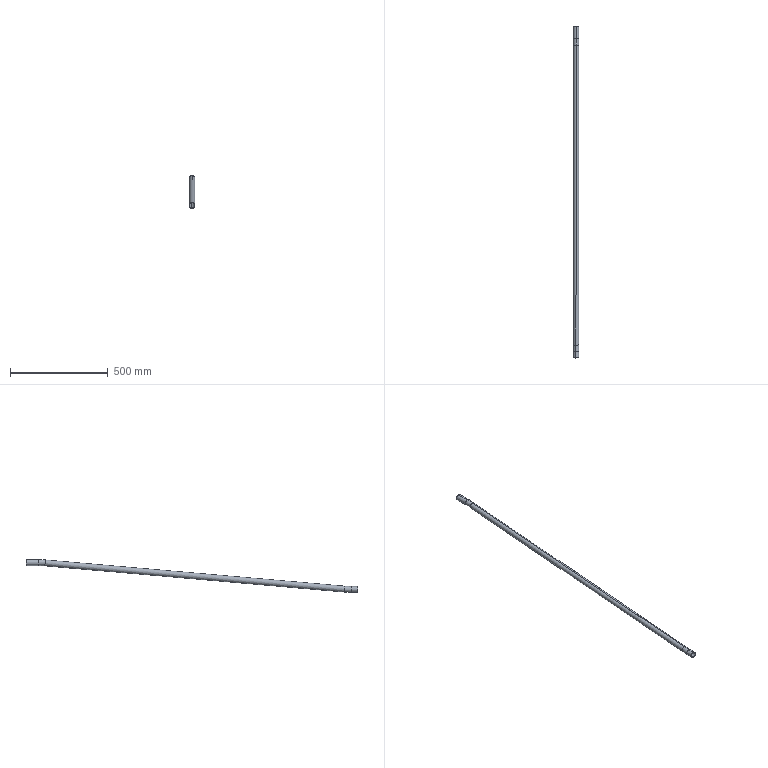Part | SolidWorks | features 3DProfileFeature 2, Sweep 1 | 1 solid | 22 faces | box 30 x 1694 x 166.835 mm | volume 299072 mm3 | cylinder 12 | torus 8 | plane 2 | commonest cylinder face diameters 26 x6 30 x6
STEP:
#1=CARTESIAN_POINT('',(19403.083,757.761,-3537.503));
#2=VERTEX_POINT('',#1);
#3=CARTESIAN_POINT('',(19403.083,755.495,-3511.602));
#4=VERTEX_POINT('',#3);
#5=CARTESIAN_POINT('',(19403.083,756.628,-3524.553));
#6=DIRECTION('',(0.,-0.9962,-0.08716));
#7=DIRECTION('',(0.,-0.08716,0.9962));
#8=AXIS2_PLACEMENT_3D('',#5,#6,#7);
#9=CIRCLE('',#8,13.);
#10=EDGE_CURVE('',#2,#4,#9,.T.);
#11=ORIENTED_EDGE('',*,*,#10,.T.);
#12=CARTESIAN_POINT('',(19403.083,791.49,-3510.03));
#13=VERTEX_POINT('',#12);
#14=CARTESIAN_POINT('',(19403.083,791.49,-3923.03));
#15=DIRECTION('',(-1.,0.,0.));
#16=DIRECTION('',(0.,0.,1.));
#17=AXIS2_PLACEMENT_3D('',#14,#15,#16);
#18=CIRCLE('',#17,413.);
#19=EDGE_CURVE('',#4,#13,#18,.T.);
#20=ORIENTED_EDGE('',*,*,#19,.T.);
#21=CARTESIAN_POINT('',(19403.083,791.49,-3536.03));
#22=VERTEX_POINT('',#21);
#23=CARTESIAN_POINT('',(19403.083,791.49,-3523.03));
#24=DIRECTION('',(0.,-1.,0.));
#25=DIRECTION('',(0.,0.,-1.));
#26=AXIS2_PLACEMENT_3D('',#23,#24,#25);
#27=CIRCLE('',#26,13.);
#28=EDGE_CURVE('',#22,#13,#27,.T.);
#29=ORIENTED_EDGE('',*,*,#28,.F.);
#30=CARTESIAN_POINT('',(19403.083,791.49,-3923.03));
#31=DIRECTION('',(-1.,0.,0.));
#32=DIRECTION('',(0.,0.,1.));
#33=AXIS2_PLACEMENT_3D('',#30,#31,#32);
#34=CIRCLE('',#33,387.);
#35=EDGE_CURVE('',#2,#22,#34,.T.);
#36=ORIENTED_EDGE('',*,*,#35,.F.);
#37=EDGE_LOOP('',(#11,#20,#29,#36));
#38=FACE_OUTER_BOUND('',#37,.T.);
#39=CARTESIAN_POINT('',(19403.083,791.49,-3923.03));
#40=DIRECTION('',(-1.,0.,0.));
#41=DIRECTION('',(0.,0.,1.));
#42=AXIS2_PLACEMENT_3D('',#39,#40,#41);
#43=TOROIDAL_SURFACE('',#42,400.,13.);
#44=ADVANCED_FACE('',(#38),#43,.F.);
#45=CARTESIAN_POINT('',(19403.083,-807.464,-3646.865));
#46=VERTEX_POINT('',#45);
#47=CARTESIAN_POINT('',(19403.083,-807.464,-3672.865));
#48=VERTEX_POINT('',#47);
#49=CARTESIAN_POINT('',(19403.083,-807.464,-3659.865));
#50=DIRECTION('',(0.,-1.,0.));
#51=DIRECTION('',(0.,0.,1.));
#52=AXIS2_PLACEMENT_3D('',#49,#50,#51);
#53=CIRCLE('',#52,13.);
#54=EDGE_CURVE('',#46,#48,#53,.T.);
#55=ORIENTED_EDGE('',*,*,#54,.T.);
#56=CARTESIAN_POINT('',(19403.083,-771.469,-3671.293));
#57=VERTEX_POINT('',#56);
#58=CARTESIAN_POINT('',(19403.083,-807.464,-3259.865));
#59=DIRECTION('',(1.,0.,0.));
#60=DIRECTION('',(0.,1.,0.));
#61=AXIS2_PLACEMENT_3D('',#58,#59,#60);
#62=CIRCLE('',#61,413.);
#63=EDGE_CURVE('',#48,#57,#62,.T.);
#64=ORIENTED_EDGE('',*,*,#63,.T.);
#65=CARTESIAN_POINT('',(19403.083,-773.735,-3645.392));
#66=VERTEX_POINT('',#65);
#67=CARTESIAN_POINT('',(19403.083,-772.602,-3658.343));
#68=DIRECTION('',(0.,-0.9962,-0.08716));
#69=DIRECTION('',(0.,0.08716,-0.9962));
#70=AXIS2_PLACEMENT_3D('',#67,#68,#69);
#71=CIRCLE('',#70,13.);
#72=EDGE_CURVE('',#66,#57,#71,.T.);
#73=ORIENTED_EDGE('',*,*,#72,.F.);
#74=CARTESIAN_POINT('',(19403.083,-807.464,-3259.865));
#75=DIRECTION('',(1.,0.,0.));
#76=DIRECTION('',(0.,1.,0.));
#77=AXIS2_PLACEMENT_3D('',#74,#75,#76);
#78=CIRCLE('',#77,387.);
#79=EDGE_CURVE('',#46,#66,#78,.T.);
#80=ORIENTED_EDGE('',*,*,#79,.F.);
#81=EDGE_LOOP('',(#55,#64,#73,#80));
#82=FACE_OUTER_BOUND('',#81,.T.);
#83=CARTESIAN_POINT('',(19403.083,-807.464,-3259.865));
#84=DIRECTION('',(1.,0.,0.));
#85=DIRECTION('',(0.,1.,0.));
#86=AXIS2_PLACEMENT_3D('',#83,#84,#85);
#87=TOROIDAL_SURFACE('',#86,400.,13.);
#88=ADVANCED_FACE('',(#82),#87,.F.);
#89=CARTESIAN_POINT('',(19403.083,755.32,-3509.61));
#90=VERTEX_POINT('',#89);
#91=CARTESIAN_POINT('',(19403.083,757.935,-3539.495));
#92=VERTEX_POINT('',#91);
#93=CARTESIAN_POINT('',(19403.083,756.628,-3524.553));
#94=DIRECTION('',(0.,-0.9962,-0.08716));
#95=DIRECTION('',(0.,0.08716,-0.9962));
#96=AXIS2_PLACEMENT_3D('',#93,#94,#95);
#97=CIRCLE('',#96,15.);
#98=EDGE_CURVE('',#90,#92,#97,.T.);
#99=ORIENTED_EDGE('',*,*,#98,.F.);
#100=CARTESIAN_POINT('',(19403.083,791.49,-3508.03));
#101=VERTEX_POINT('',#100);
#102=CARTESIAN_POINT('',(19403.083,791.49,-3923.03));
#103=DIRECTION('',(-1.,0.,0.));
#104=DIRECTION('',(0.,0.,1.));
#105=AXIS2_PLACEMENT_3D('',#102,#103,#104);
#106=CIRCLE('',#105,415.);
#107=EDGE_CURVE('',#90,#101,#106,.T.);
#108=ORIENTED_EDGE('',*,*,#107,.T.);
#109=CARTESIAN_POINT('',(19403.083,791.49,-3538.03));
#110=VERTEX_POINT('',#109);
#111=CARTESIAN_POINT('',(19403.083,791.49,-3523.03));
#112=DIRECTION('',(0.,-1.,0.));
#113=DIRECTION('',(0.,0.,-1.));
#114=AXIS2_PLACEMENT_3D('',#111,#112,#113);
#115=CIRCLE('',#114,15.);
#116=EDGE_CURVE('',#101,#110,#115,.T.);
#117=ORIENTED_EDGE('',*,*,#116,.T.);
#118=CARTESIAN_POINT('',(19403.083,791.49,-3923.03));
#119=DIRECTION('',(-1.,0.,0.));
#120=DIRECTION('',(0.,0.,1.));
#121=AXIS2_PLACEMENT_3D('',#118,#119,#120);
#122=CIRCLE('',#121,385.);
#123=EDGE_CURVE('',#92,#110,#122,.T.);
#124=ORIENTED_EDGE('',*,*,#123,.F.);
#125=EDGE_LOOP('',(#99,#108,#117,#124));
#126=FACE_OUTER_BOUND('',#125,.T.);
#127=CARTESIAN_POINT('',(19403.083,791.49,-3923.03));
#128=DIRECTION('',(-1.,0.,0.));
#129=DIRECTION('',(0.,0.,1.));
#130=AXIS2_PLACEMENT_3D('',#127,#128,#129);
#131=TOROIDAL_SURFACE('',#130,400.,15.);
#132=ADVANCED_FACE('',(#126),#131,.T.);
#133=CARTESIAN_POINT('',(19403.083,-807.464,-3674.865));
#134=VERTEX_POINT('',#133);
#135=CARTESIAN_POINT('',(19403.083,-807.464,-3644.865));
#136=VERTEX_POINT('',#135);
#137=CARTESIAN_POINT('',(19403.083,-807.464,-3659.865));
#138=DIRECTION('',(0.,-1.,0.));
#139=DIRECTION('',(0.,0.,-1.));
#140=AXIS2_PLACEMENT_3D('',#137,#138,#139);
#141=CIRCLE('',#140,15.);
#142=EDGE_CURVE('',#134,#136,#141,.T.);
#143=ORIENTED_EDGE('',*,*,#142,.F.);
#144=CARTESIAN_POINT('',(19403.083,-771.295,-3673.286));
#145=VERTEX_POINT('',#144);
#146=CARTESIAN_POINT('',(19403.083,-807.464,-3259.865));
#147=DIRECTION('',(1.,0.,0.));
#148=DIRECTION('',(0.,1.,0.));
#149=AXIS2_PLACEMENT_3D('',#146,#147,#148);
#150=CIRCLE('',#149,415.);
#151=EDGE_CURVE('',#134,#145,#150,.T.);
#152=ORIENTED_EDGE('',*,*,#151,.T.);
#153=CARTESIAN_POINT('',(19403.083,-773.909,-3643.4));
#154=VERTEX_POINT('',#153);
#155=CARTESIAN_POINT('',(19403.083,-772.602,-3658.343));
#156=DIRECTION('',(0.,-0.9962,-0.08716));
#157=DIRECTION('',(0.,0.08716,-0.9962));
#158=AXIS2_PLACEMENT_3D('',#155,#156,#157);
#159=CIRCLE('',#158,15.);
#160=EDGE_CURVE('',#145,#154,#159,.T.);
#161=ORIENTED_EDGE('',*,*,#160,.T.);
#162=CARTESIAN_POINT('',(19403.083,-807.464,-3259.865));
#163=DIRECTION('',(1.,0.,0.));
#164=DIRECTION('',(0.,1.,0.));
#165=AXIS2_PLACEMENT_3D('',#162,#163,#164);
#166=CIRCLE('',#165,385.);
#167=EDGE_CURVE('',#136,#154,#166,.T.);
#168=ORIENTED_EDGE('',*,*,#167,.F.);
#169=EDGE_LOOP('',(#143,#152,#161,#168));
#170=FACE_OUTER_BOUND('',#169,.T.);
#171=CARTESIAN_POINT('',(19403.083,-807.464,-3259.865));
#172=DIRECTION('',(1.,0.,0.));
#173=DIRECTION('',(0.,1.,0.));
#174=AXIS2_PLACEMENT_3D('',#171,#172,#173);
#175=TOROIDAL_SURFACE('',#174,400.,15.);
#176=ADVANCED_FACE('',(#170),#175,.T.);
#177=CARTESIAN_POINT('',(19403.083,791.49,-3523.03));
#178=DIRECTION('',(0.,-1.,0.));
#179=DIRECTION('',(0.,0.,-1.));
#180=AXIS2_PLACEMENT_3D('',#177,#178,#179);
#181=CIRCLE('',#180,13.);
#182=EDGE_CURVE('',#13,#22,#181,.T.);
#183=ORIENTED_EDGE('',*,*,#182,.T.);
#184=CARTESIAN_POINT('',(19403.083,854.026,-3536.03));
#185=VERTEX_POINT('',#184);
#186=CARTESIAN_POINT('',(19403.083,791.49,-3536.03));
#187=DIRECTION('',(0.,1.,0.));
#188=VECTOR('',#187,1000.);
#189=LINE('',#186,#188);
#190=EDGE_CURVE('',#22,#185,#189,.T.);
#191=ORIENTED_EDGE('',*,*,#190,.T.);
#192=CARTESIAN_POINT('',(19403.083,854.026,-3510.03));
#193=VERTEX_POINT('',#192);
#194=CARTESIAN_POINT('',(19403.083,854.026,-3523.03));
#195=DIRECTION('',(0.,-1.,0.));
#196=DIRECTION('',(0.,0.,-1.));
#197=AXIS2_PLACEMENT_3D('',#194,#195,#196);
#198=CIRCLE('',#197,13.);
#199=EDGE_CURVE('',#193,#185,#198,.T.);
#200=ORIENTED_EDGE('',*,*,#199,.F.);
#201=CARTESIAN_POINT('',(19403.083,791.49,-3510.03));
#202=DIRECTION('',(0.,1.,0.));
#203=VECTOR('',#202,1000.);
#204=LINE('',#201,#203);
#205=EDGE_CURVE('',#13,#193,#204,.T.);
#206=ORIENTED_EDGE('',*,*,#205,.F.);
#207=EDGE_LOOP('',(#183,#191,#200,#206));
#208=FACE_OUTER_BOUND('',#207,.T.);
#209=CARTESIAN_POINT('',(19403.083,791.49,-3523.03));
#210=DIRECTION('',(0.,1.,0.));
#211=DIRECTION('',(0.,0.,1.));
#212=AXIS2_PLACEMENT_3D('',#209,#210,#211);
#213=CYLINDRICAL_SURFACE('',#212,13.);
#214=ADVANCED_FACE('',(#208),#213,.F.);
#215=ORIENTED_EDGE('',*,*,#72,.T.);
#216=CARTESIAN_POINT('',(19403.083,-771.469,-3671.293));
#217=DIRECTION('',(0.,0.9962,0.08716));
#218=VECTOR('',#217,1000.);
#219=LINE('',#216,#218);
#220=EDGE_CURVE('',#57,#2,#219,.T.);
#221=ORIENTED_EDGE('',*,*,#220,.T.);
#222=CARTESIAN_POINT('',(19403.083,756.628,-3524.553));
#223=DIRECTION('',(0.,-0.9962,-0.08716));
#224=DIRECTION('',(0.,-0.08716,0.9962));
#225=AXIS2_PLACEMENT_3D('',#222,#223,#224);
#226=CIRCLE('',#225,13.);
#227=EDGE_CURVE('',#4,#2,#226,.T.);
#228=ORIENTED_EDGE('',*,*,#227,.F.);
#229=CARTESIAN_POINT('',(19403.083,-773.735,-3645.392));
#230=DIRECTION('',(0.,0.9962,0.08716));
#231=VECTOR('',#230,1000.);
#232=LINE('',#229,#231);
#233=EDGE_CURVE('',#66,#4,#232,.T.);
#234=ORIENTED_EDGE('',*,*,#233,.F.);
#235=EDGE_LOOP('',(#215,#221,#228,#234));
#236=FACE_OUTER_BOUND('',#235,.T.);
#237=CARTESIAN_POINT('',(19403.083,-772.602,-3658.343));
#238=DIRECTION('',(0.,0.9962,0.08716));
#239=DIRECTION('',(0.,-0.08716,0.9962));
#240=AXIS2_PLACEMENT_3D('',#237,#238,#239);
#241=CYLINDRICAL_SURFACE('',#240,13.);
#242=ADVANCED_FACE('',(#236),#241,.F.);
#243=CARTESIAN_POINT('',(19403.083,-840.,-3646.865));
#244=VERTEX_POINT('',#243);
#245=CARTESIAN_POINT('',(19403.083,-840.,-3672.865));
#246=VERTEX_POINT('',#245);
#247=CARTESIAN_POINT('',(19403.083,-840.,-3659.865));
#248=DIRECTION('',(0.,-1.,0.));
#249=DIRECTION('',(0.,0.,-1.));
#250=AXIS2_PLACEMENT_3D('',#247,#248,#249);
#251=CIRCLE('',#250,13.);
#252=EDGE_CURVE('',#244,#246,#251,.T.);
#253=ORIENTED_EDGE('',*,*,#252,.T.);
#254=CARTESIAN_POINT('',(19403.083,-840.,-3672.865));
#255=DIRECTION('',(0.,1.,0.));
#256=VECTOR('',#255,1000.);
#257=LINE('',#254,#256);
#258=EDGE_CURVE('',#246,#48,#257,.T.);
#259=ORIENTED_EDGE('',*,*,#258,.T.);
#260=ORIENTED_EDGE('',*,*,#54,.F.);
#261=CARTESIAN_POINT('',(19403.083,-840.,-3646.865));
#262=DIRECTION('',(0.,1.,0.));
#263=VECTOR('',#262,1000.);
#264=LINE('',#261,#263);
#265=EDGE_CURVE('',#244,#46,#264,.T.);
#266=ORIENTED_EDGE('',*,*,#265,.F.);
#267=EDGE_LOOP('',(#253,#259,#260,#266));
#268=FACE_OUTER_BOUND('',#267,.T.);
#269=CARTESIAN_POINT('',(19403.083,-840.,-3659.865));
#270=DIRECTION('',(0.,1.,0.));
#271=DIRECTION('',(0.,0.,1.));
#272=AXIS2_PLACEMENT_3D('',#269,#270,#271);
#273=CYLINDRICAL_SURFACE('',#272,13.);
#274=ADVANCED_FACE('',(#268),#273,.F.);
#275=CARTESIAN_POINT('',(19403.083,791.49,-3523.03));
#276=DIRECTION('',(0.,-1.,0.));
#277=DIRECTION('',(0.,0.,-1.));
#278=AXIS2_PLACEMENT_3D('',#275,#276,#277);
#279=CIRCLE('',#278,15.);
#280=EDGE_CURVE('',#110,#101,#279,.T.);
#281=ORIENTED_EDGE('',*,*,#280,.F.);
#282=CARTESIAN_POINT('',(19403.083,854.026,-3538.03));
#283=VERTEX_POINT('',#282);
#284=CARTESIAN_POINT('',(19403.083,791.49,-3538.03));
#285=DIRECTION('',(0.,1.,0.));
#286=VECTOR('',#285,1000.);
#287=LINE('',#284,#286);
#288=EDGE_CURVE('',#110,#283,#287,.T.);
#289=ORIENTED_EDGE('',*,*,#288,.T.);
#290=CARTESIAN_POINT('',(19403.083,854.026,-3508.03));
#291=VERTEX_POINT('',#290);
#292=CARTESIAN_POINT('',(19403.083,854.026,-3523.03));
#293=DIRECTION('',(0.,-1.,0.));
#294=DIRECTION('',(0.,0.,-1.));
#295=AXIS2_PLACEMENT_3D('',#292,#293,#294);
#296=CIRCLE('',#295,15.);
#297=EDGE_CURVE('',#283,#291,#296,.T.);
#298=ORIENTED_EDGE('',*,*,#297,.T.);
#299=CARTESIAN_POINT('',(19403.083,791.49,-3508.03));
#300=DIRECTION('',(0.,1.,0.));
#301=VECTOR('',#300,1000.);
#302=LINE('',#299,#301);
#303=EDGE_CURVE('',#101,#291,#302,.T.);
#304=ORIENTED_EDGE('',*,*,#303,.F.);
#305=EDGE_LOOP('',(#281,#289,#298,#304));
#306=FACE_OUTER_BOUND('',#305,.T.);
#307=CARTESIAN_POINT('',(19403.083,791.49,-3523.03));
#308=DIRECTION('',(0.,1.,0.));
#309=DIRECTION('',(0.,0.,1.));
#310=AXIS2_PLACEMENT_3D('',#307,#308,#309);
#311=CYLINDRICAL_SURFACE('',#310,15.);
#312=ADVANCED_FACE('',(#306),#311,.T.);
#313=ORIENTED_EDGE('',*,*,#160,.F.);
#314=CARTESIAN_POINT('',(19403.083,-771.295,-3673.286));
#315=DIRECTION('',(0.,0.9962,0.08716));
#316=VECTOR('',#315,1000.);
#317=LINE('',#314,#316);
#318=EDGE_CURVE('',#145,#92,#317,.T.);
#319=ORIENTED_EDGE('',*,*,#318,.T.);
#320=CARTESIAN_POINT('',(19403.083,756.628,-3524.553));
#321=DIRECTION('',(0.,-0.9962,-0.08716));
#322=DIRECTION('',(0.,0.08716,-0.9962));
#323=AXIS2_PLACEMENT_3D('',#320,#321,#322);
#324=CIRCLE('',#323,15.);
#325=EDGE_CURVE('',#92,#90,#324,.T.);
#326=ORIENTED_EDGE('',*,*,#325,.T.);
#327=CARTESIAN_POINT('',(19403.083,-773.909,-3643.4));
#328=DIRECTION('',(0.,0.9962,0.08716));
#329=VECTOR('',#328,1000.);
#330=LINE('',#327,#329);
#331=EDGE_CURVE('',#154,#90,#330,.T.);
#332=ORIENTED_EDGE('',*,*,#331,.F.);
#333=EDGE_LOOP('',(#313,#319,#326,#332));
#334=FACE_OUTER_BOUND('',#333,.T.);
#335=CARTESIAN_POINT('',(19403.083,-772.602,-3658.343));
#336=DIRECTION('',(0.,0.9962,0.08716));
#337=DIRECTION('',(0.,-0.08716,0.9962));
#338=AXIS2_PLACEMENT_3D('',#335,#336,#337);
#339=CYLINDRICAL_SURFACE('',#338,15.);
#340=ADVANCED_FACE('',(#334),#339,.T.);
#341=CARTESIAN_POINT('',(19403.083,-840.,-3674.865));
#342=VERTEX_POINT('',#341);
#343=CARTESIAN_POINT('',(19403.083,-840.,-3644.865));
#344=VERTEX_POINT('',#343);
#345=CARTESIAN_POINT('',(19403.083,-840.,-3659.865));
#346=DIRECTION('',(0.,-1.,0.));
#347=DIRECTION('',(0.,0.,-1.));
#348=AXIS2_PLACEMENT_3D('',#345,#346,#347);
#349=CIRCLE('',#348,15.);
#350=EDGE_CURVE('',#342,#344,#349,.T.);
#351=ORIENTED_EDGE('',*,*,#350,.F.);
#352=CARTESIAN_POINT('',(19403.083,-840.,-3674.865));
#353=DIRECTION('',(0.,1.,0.));
#354=VECTOR('',#353,1000.);
#355=LINE('',#352,#354);
#356=EDGE_CURVE('',#342,#134,#355,.T.);
#357=ORIENTED_EDGE('',*,*,#356,.T.);
#358=ORIENTED_EDGE('',*,*,#142,.T.);
#359=CARTESIAN_POINT('',(19403.083,-840.,-3644.865));
#360=DIRECTION('',(0.,1.,0.));
#361=VECTOR('',#360,1000.);
#362=LINE('',#359,#361);
#363=EDGE_CURVE('',#344,#136,#362,.T.);
#364=ORIENTED_EDGE('',*,*,#363,.F.);
#365=EDGE_LOOP('',(#351,#357,#358,#364));
#366=FACE_OUTER_BOUND('',#365,.T.);
#367=CARTESIAN_POINT('',(19403.083,-840.,-3659.865));
#368=DIRECTION('',(0.,1.,0.));
#369=DIRECTION('',(0.,0.,1.));
#370=AXIS2_PLACEMENT_3D('',#367,#368,#369);
#371=CYLINDRICAL_SURFACE('',#370,15.);
#372=ADVANCED_FACE('',(#366),#371,.T.);
#373=ORIENTED_EDGE('',*,*,#288,.F.);
#374=ORIENTED_EDGE('',*,*,#116,.F.);
#375=ORIENTED_EDGE('',*,*,#303,.T.);
#376=CARTESIAN_POINT('',(19403.083,854.026,-3523.03));
#377=DIRECTION('',(0.,-1.,0.));
#378=DIRECTION('',(0.,0.,-1.));
#379=AXIS2_PLACEMENT_3D('',#376,#377,#378);
#380=CIRCLE('',#379,15.);
#381=EDGE_CURVE('',#291,#283,#380,.T.);
#382=ORIENTED_EDGE('',*,*,#381,.T.);
#383=EDGE_LOOP('',(#373,#374,#375,#382));
#384=FACE_OUTER_BOUND('',#383,.T.);
#385=CARTESIAN_POINT('',(19403.083,791.49,-3523.03));
#386=DIRECTION('',(0.,1.,0.));
#387=DIRECTION('',(0.,0.,1.));
#388=AXIS2_PLACEMENT_3D('',#385,#386,#387);
#389=CYLINDRICAL_SURFACE('',#388,15.);
#390=ADVANCED_FACE('',(#384),#389,.T.);
#391=ORIENTED_EDGE('',*,*,#107,.F.);
#392=ORIENTED_EDGE('',*,*,#325,.F.);
#393=ORIENTED_EDGE('',*,*,#123,.T.);
#394=ORIENTED_EDGE('',*,*,#280,.T.);
#395=EDGE_LOOP('',(#391,#392,#393,#394));
#396=FACE_OUTER_BOUND('',#395,.T.);
#397=CARTESIAN_POINT('',(19403.083,791.49,-3923.03));
#398=DIRECTION('',(-1.,0.,0.));
#399=DIRECTION('',(0.,0.,1.));
#400=AXIS2_PLACEMENT_3D('',#397,#398,#399);
#401=TOROIDAL_SURFACE('',#400,400.,15.);
#402=ADVANCED_FACE('',(#396),#401,.T.);
#403=ORIENTED_EDGE('',*,*,#318,.F.);
#404=CARTESIAN_POINT('',(19403.083,-772.602,-3658.343));
#405=DIRECTION('',(0.,-0.9962,-0.08716));
#406=DIRECTION('',(0.,0.08716,-0.9962));
#407=AXIS2_PLACEMENT_3D('',#404,#405,#406);
#408=CIRCLE('',#407,15.);
#409=EDGE_CURVE('',#154,#145,#408,.T.);
#410=ORIENTED_EDGE('',*,*,#409,.F.);
#411=ORIENTED_EDGE('',*,*,#331,.T.);
#412=ORIENTED_EDGE('',*,*,#98,.T.);
#413=EDGE_LOOP('',(#403,#410,#411,#412));
#414=FACE_OUTER_BOUND('',#413,.T.);
#415=CARTESIAN_POINT('',(19403.083,-772.602,-3658.343));
#416=DIRECTION('',(0.,0.9962,0.08716));
#417=DIRECTION('',(0.,-0.08716,0.9962));
#418=AXIS2_PLACEMENT_3D('',#415,#416,#417);
#419=CYLINDRICAL_SURFACE('',#418,15.);
#420=ADVANCED_FACE('',(#414),#419,.T.);
#421=ORIENTED_EDGE('',*,*,#151,.F.);
#422=CARTESIAN_POINT('',(19403.083,-807.464,-3659.865));
#423=DIRECTION('',(0.,-1.,0.));
#424=DIRECTION('',(0.,0.,-1.));
#425=AXIS2_PLACEMENT_3D('',#422,#423,#424);
#426=CIRCLE('',#425,15.);
#427=EDGE_CURVE('',#136,#134,#426,.T.);
#428=ORIENTED_EDGE('',*,*,#427,.F.);
#429=ORIENTED_EDGE('',*,*,#167,.T.);
#430=ORIENTED_EDGE('',*,*,#409,.T.);
#431=EDGE_LOOP('',(#421,#428,#429,#430));
#432=FACE_OUTER_BOUND('',#431,.T.);
#433=CARTESIAN_POINT('',(19403.083,-807.464,-3259.865));
#434=DIRECTION('',(1.,0.,0.));
#435=DIRECTION('',(0.,1.,0.));
#436=AXIS2_PLACEMENT_3D('',#433,#434,#435);
#437=TOROIDAL_SURFACE('',#436,400.,15.);
#438=ADVANCED_FACE('',(#432),#437,.T.);
#439=ORIENTED_EDGE('',*,*,#356,.F.);
#440=CARTESIAN_POINT('',(19403.083,-840.,-3659.865));
#441=DIRECTION('',(0.,-1.,0.));
#442=DIRECTION('',(0.,0.,-1.));
#443=AXIS2_PLACEMENT_3D('',#440,#441,#442);
#444=CIRCLE('',#443,15.);
#445=EDGE_CURVE('',#344,#342,#444,.T.);
#446=ORIENTED_EDGE('',*,*,#445,.F.);
#447=ORIENTED_EDGE('',*,*,#363,.T.);
#448=ORIENTED_EDGE('',*,*,#427,.T.);
#449=EDGE_LOOP('',(#439,#446,#447,#448));
#450=FACE_OUTER_BOUND('',#449,.T.);
#451=CARTESIAN_POINT('',(19403.083,-840.,-3659.865));
#452=DIRECTION('',(0.,1.,0.));
#453=DIRECTION('',(0.,0.,1.));
#454=AXIS2_PLACEMENT_3D('',#451,#452,#453);
#455=CYLINDRICAL_SURFACE('',#454,15.);
#456=ADVANCED_FACE('',(#450),#455,.T.);
#457=ORIENTED_EDGE('',*,*,#199,.T.);
#458=CARTESIAN_POINT('',(19403.083,854.026,-3523.03));
#459=DIRECTION('',(0.,-1.,0.));
#460=DIRECTION('',(0.,0.,-1.));
#461=AXIS2_PLACEMENT_3D('',#458,#459,#460);
#462=CIRCLE('',#461,13.);
#463=EDGE_CURVE('',#185,#193,#462,.T.);
#464=ORIENTED_EDGE('',*,*,#463,.T.);
#465=EDGE_LOOP('',(#457,#464));
#466=FACE_BOUND('',#465,.T.);
#467=ORIENTED_EDGE('',*,*,#381,.F.);
#468=ORIENTED_EDGE('',*,*,#297,.F.);
#469=EDGE_LOOP('',(#467,#468));
#470=FACE_OUTER_BOUND('',#469,.T.);
#471=CARTESIAN_POINT('',(19403.083,854.026,-3523.03));
#472=DIRECTION('',(0.,-1.,0.));
#473=DIRECTION('',(0.,0.,-1.));
#474=AXIS2_PLACEMENT_3D('',#471,#472,#473);
#475=PLANE('',#474);
#476=ADVANCED_FACE('',(#466,#470),#475,.F.);
#477=ORIENTED_EDGE('',*,*,#252,.F.);
#478=CARTESIAN_POINT('',(19403.083,-840.,-3659.865));
#479=DIRECTION('',(0.,-1.,0.));
#480=DIRECTION('',(0.,0.,-1.));
#481=AXIS2_PLACEMENT_3D('',#478,#479,#480);
#482=CIRCLE('',#481,13.);
#483=EDGE_CURVE('',#246,#244,#482,.T.);
#484=ORIENTED_EDGE('',*,*,#483,.F.);
#485=EDGE_LOOP('',(#477,#484));
#486=FACE_BOUND('',#485,.T.);
#487=ORIENTED_EDGE('',*,*,#445,.T.);
#488=ORIENTED_EDGE('',*,*,#350,.T.);
#489=EDGE_LOOP('',(#487,#488));
#490=FACE_OUTER_BOUND('',#489,.T.);
#491=CARTESIAN_POINT('',(19403.083,-840.,-3659.865));
#492=DIRECTION('',(0.,-1.,0.));
#493=DIRECTION('',(0.,0.,-1.));
#494=AXIS2_PLACEMENT_3D('',#491,#492,#493);
#495=PLANE('',#494);
#496=ADVANCED_FACE('',(#486,#490),#495,.T.);
#497=ORIENTED_EDGE('',*,*,#190,.F.);
#498=ORIENTED_EDGE('',*,*,#28,.T.);
#499=ORIENTED_EDGE('',*,*,#205,.T.);
#500=ORIENTED_EDGE('',*,*,#463,.F.);
#501=EDGE_LOOP('',(#497,#498,#499,#500));
#502=FACE_OUTER_BOUND('',#501,.T.);
#503=CARTESIAN_POINT('',(19403.083,791.49,-3523.03));
#504=DIRECTION('',(0.,1.,0.));
#505=DIRECTION('',(0.,0.,1.));
#506=AXIS2_PLACEMENT_3D('',#503,#504,#505);
#507=CYLINDRICAL_SURFACE('',#506,13.);
#508=ADVANCED_FACE('',(#502),#507,.F.);
#509=ORIENTED_EDGE('',*,*,#19,.F.);
#510=ORIENTED_EDGE('',*,*,#227,.T.);
#511=ORIENTED_EDGE('',*,*,#35,.T.);
#512=ORIENTED_EDGE('',*,*,#182,.F.);
#513=EDGE_LOOP('',(#509,#510,#511,#512));
#514=FACE_OUTER_BOUND('',#513,.T.);
#515=CARTESIAN_POINT('',(19403.083,791.49,-3923.03));
#516=DIRECTION('',(-1.,0.,0.));
#517=DIRECTION('',(0.,0.,1.));
#518=AXIS2_PLACEMENT_3D('',#515,#516,#517);
#519=TOROIDAL_SURFACE('',#518,400.,13.);
#520=ADVANCED_FACE('',(#514),#519,.F.);
#521=ORIENTED_EDGE('',*,*,#220,.F.);
#522=CARTESIAN_POINT('',(19403.083,-772.602,-3658.343));
#523=DIRECTION('',(0.,-0.9962,-0.08716));
#524=DIRECTION('',(0.,0.08716,-0.9962));
#525=AXIS2_PLACEMENT_3D('',#522,#523,#524);
#526=CIRCLE('',#525,13.);
#527=EDGE_CURVE('',#57,#66,#526,.T.);
#528=ORIENTED_EDGE('',*,*,#527,.T.);
#529=ORIENTED_EDGE('',*,*,#233,.T.);
#530=ORIENTED_EDGE('',*,*,#10,.F.);
#531=EDGE_LOOP('',(#521,#528,#529,#530));
#532=FACE_OUTER_BOUND('',#531,.T.);
#533=CARTESIAN_POINT('',(19403.083,-772.602,-3658.343));
#534=DIRECTION('',(0.,0.9962,0.08716));
#535=DIRECTION('',(0.,-0.08716,0.9962));
#536=AXIS2_PLACEMENT_3D('',#533,#534,#535);
#537=CYLINDRICAL_SURFACE('',#536,13.);
#538=ADVANCED_FACE('',(#532),#537,.F.);
#539=ORIENTED_EDGE('',*,*,#63,.F.);
#540=CARTESIAN_POINT('',(19403.083,-807.464,-3659.865));
#541=DIRECTION('',(0.,-1.,0.));
#542=DIRECTION('',(0.,0.,1.));
#543=AXIS2_PLACEMENT_3D('',#540,#541,#542);
#544=CIRCLE('',#543,13.);
#545=EDGE_CURVE('',#48,#46,#544,.T.);
#546=ORIENTED_EDGE('',*,*,#545,.T.);
#547=ORIENTED_EDGE('',*,*,#79,.T.);
#548=ORIENTED_EDGE('',*,*,#527,.F.);
#549=EDGE_LOOP('',(#539,#546,#547,#548));
#550=FACE_OUTER_BOUND('',#549,.T.);
#551=CARTESIAN_POINT('',(19403.083,-807.464,-3259.865));
#552=DIRECTION('',(1.,0.,0.));
#553=DIRECTION('',(0.,1.,0.));
#554=AXIS2_PLACEMENT_3D('',#551,#552,#553);
#555=TOROIDAL_SURFACE('',#554,400.,13.);
#556=ADVANCED_FACE('',(#550),#555,.F.);
#557=ORIENTED_EDGE('',*,*,#258,.F.);
#558=ORIENTED_EDGE('',*,*,#483,.T.);
#559=ORIENTED_EDGE('',*,*,#265,.T.);
#560=ORIENTED_EDGE('',*,*,#545,.F.);
#561=EDGE_LOOP('',(#557,#558,#559,#560));
#562=FACE_OUTER_BOUND('',#561,.T.);
#563=CARTESIAN_POINT('',(19403.083,-840.,-3659.865));
#564=DIRECTION('',(0.,1.,0.));
#565=DIRECTION('',(0.,0.,1.));
#566=AXIS2_PLACEMENT_3D('',#563,#564,#565);
#567=CYLINDRICAL_SURFACE('',#566,13.);
#568=ADVANCED_FACE('',(#562),#567,.F.);
#569=CLOSED_SHELL('',(#44,#88,#132,#176,#214,#242,#274,#312,#340,#372,#390,#402,#420,#438,#456,#476,#496,#508,#520,#538,#556,#568));
#570=MANIFOLD_SOLID_BREP('',#569);
#571=CARTESIAN_POINT('',(0.,0.,0.));
#572=DIRECTION('',(0.,0.,1.));
#573=DIRECTION('',(1.,0.,0.));
#574=AXIS2_PLACEMENT_3D('',#571,#572,#573);
#575=(LENGTH_UNIT()NAMED_UNIT(*)SI_UNIT(.MILLI.,.METRE.));
#576=UNCERTAINTY_MEASURE_WITH_UNIT(LENGTH_MEASURE(0.00001),#575,'','');
#577=(NAMED_UNIT(*)PLANE_ANGLE_UNIT()SI_UNIT($,.RADIAN.));
#578=(NAMED_UNIT(*)SI_UNIT($,.STERADIAN.)SOLID_ANGLE_UNIT());
#579=(GEOMETRIC_REPRESENTATION_CONTEXT(3)GLOBAL_UNCERTAINTY_ASSIGNED_CONTEXT((#576))GLOBAL_UNIT_ASSIGNED_CONTEXT((#575,#577,#578))REPRESENTATION_CONTEXT('',''));
#580=ADVANCED_BREP_SHAPE_REPRESENTATION('',(#570,#574),#579);